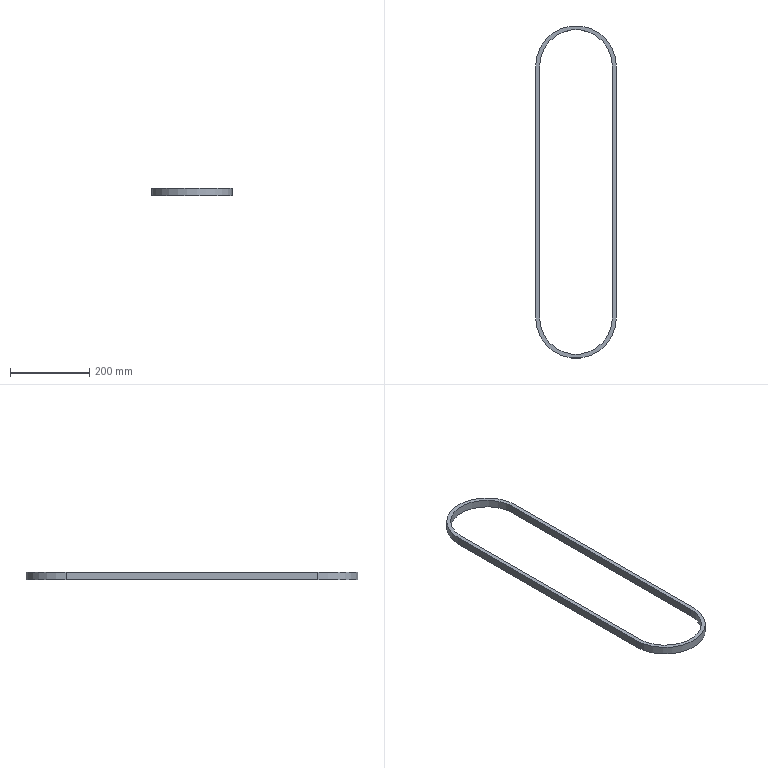Part | SolidWorks | features BeltProfileFeature 1, ExtruThin 1 | 1 solid | 10 faces | box 203.25 x 838.25 x 20 mm | volume 375423 mm3 | plane 6 | cylinder 4 | commonest cylinder face diameters 183.25 x2 203.25 x2
STEP:
#1=CARTESIAN_POINT('',(101.625,0.,10.));
#2=VERTEX_POINT('',#1);
#3=CARTESIAN_POINT('',(-101.625,0.,10.));
#4=VERTEX_POINT('',#3);
#5=CARTESIAN_POINT('',(0.,0.,10.));
#6=DIRECTION('',(0.,0.,1.));
#7=DIRECTION('',(-1.,0.,0.));
#8=AXIS2_PLACEMENT_3D('',#5,#6,#7);
#9=CIRCLE('',#8,101.625);
#10=EDGE_CURVE('',#2,#4,#9,.T.);
#11=ORIENTED_EDGE('',*,*,#10,.T.);
#12=CARTESIAN_POINT('',(-101.625,-635.,10.));
#13=VERTEX_POINT('',#12);
#14=CARTESIAN_POINT('',(-101.625,0.,10.));
#15=DIRECTION('',(0.,-1.,0.));
#16=VECTOR('',#15,1000.);
#17=LINE('',#14,#16);
#18=EDGE_CURVE('',#4,#13,#17,.T.);
#19=ORIENTED_EDGE('',*,*,#18,.T.);
#20=CARTESIAN_POINT('',(101.625,-635.,10.));
#21=VERTEX_POINT('',#20);
#22=CARTESIAN_POINT('',(0.,-635.,10.));
#23=DIRECTION('',(0.,0.,1.));
#24=DIRECTION('',(-1.,0.,0.));
#25=AXIS2_PLACEMENT_3D('',#22,#23,#24);
#26=CIRCLE('',#25,101.625);
#27=EDGE_CURVE('',#13,#21,#26,.T.);
#28=ORIENTED_EDGE('',*,*,#27,.T.);
#29=CARTESIAN_POINT('',(101.625,0.,10.));
#30=DIRECTION('',(0.,1.,0.));
#31=VECTOR('',#30,1000.);
#32=LINE('',#29,#31);
#33=EDGE_CURVE('',#21,#2,#32,.T.);
#34=ORIENTED_EDGE('',*,*,#33,.T.);
#35=EDGE_LOOP('',(#11,#19,#28,#34));
#36=FACE_OUTER_BOUND('',#35,.T.);
#37=CARTESIAN_POINT('',(91.625,0.,10.));
#38=VERTEX_POINT('',#37);
#39=CARTESIAN_POINT('',(-91.625,0.,10.));
#40=VERTEX_POINT('',#39);
#41=CARTESIAN_POINT('',(0.,0.,10.));
#42=DIRECTION('',(0.,0.,1.));
#43=DIRECTION('',(-1.,0.,0.));
#44=AXIS2_PLACEMENT_3D('',#41,#42,#43);
#45=CIRCLE('',#44,91.625);
#46=EDGE_CURVE('',#38,#40,#45,.T.);
#47=ORIENTED_EDGE('',*,*,#46,.F.);
#48=CARTESIAN_POINT('',(91.625,-635.,10.));
#49=VERTEX_POINT('',#48);
#50=CARTESIAN_POINT('',(91.625,0.,10.));
#51=DIRECTION('',(0.,1.,0.));
#52=VECTOR('',#51,1000.);
#53=LINE('',#50,#52);
#54=EDGE_CURVE('',#49,#38,#53,.T.);
#55=ORIENTED_EDGE('',*,*,#54,.F.);
#56=CARTESIAN_POINT('',(-91.625,-635.,10.));
#57=VERTEX_POINT('',#56);
#58=CARTESIAN_POINT('',(0.,-635.,10.));
#59=DIRECTION('',(0.,0.,1.));
#60=DIRECTION('',(-1.,0.,0.));
#61=AXIS2_PLACEMENT_3D('',#58,#59,#60);
#62=CIRCLE('',#61,91.625);
#63=EDGE_CURVE('',#57,#49,#62,.T.);
#64=ORIENTED_EDGE('',*,*,#63,.F.);
#65=CARTESIAN_POINT('',(-91.625,-635.,10.));
#66=DIRECTION('',(0.,-1.,0.));
#67=VECTOR('',#66,1000.);
#68=LINE('',#65,#67);
#69=EDGE_CURVE('',#40,#57,#68,.T.);
#70=ORIENTED_EDGE('',*,*,#69,.F.);
#71=EDGE_LOOP('',(#47,#55,#64,#70));
#72=FACE_BOUND('',#71,.T.);
#73=CARTESIAN_POINT('',(0.,0.,10.));
#74=DIRECTION('',(0.,0.,-1.));
#75=DIRECTION('',(-1.,0.,0.));
#76=AXIS2_PLACEMENT_3D('',#73,#74,#75);
#77=PLANE('',#76);
#78=ADVANCED_FACE('',(#36,#72),#77,.F.);
#79=CARTESIAN_POINT('',(101.625,0.,-10.));
#80=VERTEX_POINT('',#79);
#81=CARTESIAN_POINT('',(-101.625,0.,-10.));
#82=VERTEX_POINT('',#81);
#83=CARTESIAN_POINT('',(0.,0.,-10.));
#84=DIRECTION('',(0.,0.,1.));
#85=DIRECTION('',(-1.,0.,0.));
#86=AXIS2_PLACEMENT_3D('',#83,#84,#85);
#87=CIRCLE('',#86,101.625);
#88=EDGE_CURVE('',#80,#82,#87,.T.);
#89=ORIENTED_EDGE('',*,*,#88,.F.);
#90=CARTESIAN_POINT('',(101.625,-635.,-10.));
#91=VERTEX_POINT('',#90);
#92=CARTESIAN_POINT('',(101.625,0.,-10.));
#93=DIRECTION('',(0.,1.,0.));
#94=VECTOR('',#93,1000.);
#95=LINE('',#92,#94);
#96=EDGE_CURVE('',#91,#80,#95,.T.);
#97=ORIENTED_EDGE('',*,*,#96,.F.);
#98=CARTESIAN_POINT('',(-101.625,-635.,-10.));
#99=VERTEX_POINT('',#98);
#100=CARTESIAN_POINT('',(0.,-635.,-10.));
#101=DIRECTION('',(0.,0.,1.));
#102=DIRECTION('',(-1.,0.,0.));
#103=AXIS2_PLACEMENT_3D('',#100,#101,#102);
#104=CIRCLE('',#103,101.625);
#105=EDGE_CURVE('',#99,#91,#104,.T.);
#106=ORIENTED_EDGE('',*,*,#105,.F.);
#107=CARTESIAN_POINT('',(-101.625,0.,-10.));
#108=DIRECTION('',(0.,-1.,0.));
#109=VECTOR('',#108,1000.);
#110=LINE('',#107,#109);
#111=EDGE_CURVE('',#82,#99,#110,.T.);
#112=ORIENTED_EDGE('',*,*,#111,.F.);
#113=EDGE_LOOP('',(#89,#97,#106,#112));
#114=FACE_OUTER_BOUND('',#113,.T.);
#115=CARTESIAN_POINT('',(91.625,-635.,-10.));
#116=VERTEX_POINT('',#115);
#117=CARTESIAN_POINT('',(91.625,0.,-10.));
#118=VERTEX_POINT('',#117);
#119=CARTESIAN_POINT('',(91.625,0.,-10.));
#120=DIRECTION('',(0.,1.,0.));
#121=VECTOR('',#120,1000.);
#122=LINE('',#119,#121);
#123=EDGE_CURVE('',#116,#118,#122,.T.);
#124=ORIENTED_EDGE('',*,*,#123,.T.);
#125=CARTESIAN_POINT('',(-91.625,0.,-10.));
#126=VERTEX_POINT('',#125);
#127=CARTESIAN_POINT('',(0.,0.,-10.));
#128=DIRECTION('',(0.,0.,1.));
#129=DIRECTION('',(-1.,0.,0.));
#130=AXIS2_PLACEMENT_3D('',#127,#128,#129);
#131=CIRCLE('',#130,91.625);
#132=EDGE_CURVE('',#118,#126,#131,.T.);
#133=ORIENTED_EDGE('',*,*,#132,.T.);
#134=CARTESIAN_POINT('',(-91.625,-635.,-10.));
#135=VERTEX_POINT('',#134);
#136=CARTESIAN_POINT('',(-91.625,-635.,-10.));
#137=DIRECTION('',(0.,-1.,0.));
#138=VECTOR('',#137,1000.);
#139=LINE('',#136,#138);
#140=EDGE_CURVE('',#126,#135,#139,.T.);
#141=ORIENTED_EDGE('',*,*,#140,.T.);
#142=CARTESIAN_POINT('',(0.,-635.,-10.));
#143=DIRECTION('',(0.,0.,1.));
#144=DIRECTION('',(-1.,0.,0.));
#145=AXIS2_PLACEMENT_3D('',#142,#143,#144);
#146=CIRCLE('',#145,91.625);
#147=EDGE_CURVE('',#135,#116,#146,.T.);
#148=ORIENTED_EDGE('',*,*,#147,.T.);
#149=EDGE_LOOP('',(#124,#133,#141,#148));
#150=FACE_BOUND('',#149,.T.);
#151=CARTESIAN_POINT('',(0.,0.,-10.));
#152=DIRECTION('',(0.,0.,-1.));
#153=DIRECTION('',(-1.,0.,0.));
#154=AXIS2_PLACEMENT_3D('',#151,#152,#153);
#155=PLANE('',#154);
#156=ADVANCED_FACE('',(#114,#150),#155,.T.);
#157=ORIENTED_EDGE('',*,*,#88,.T.);
#158=CARTESIAN_POINT('',(-101.625,0.,10.));
#159=DIRECTION('',(0.,0.,-1.));
#160=VECTOR('',#159,1000.);
#161=LINE('',#158,#160);
#162=EDGE_CURVE('',#4,#82,#161,.T.);
#163=ORIENTED_EDGE('',*,*,#162,.F.);
#164=ORIENTED_EDGE('',*,*,#10,.F.);
#165=CARTESIAN_POINT('',(101.625,0.,10.));
#166=DIRECTION('',(0.,0.,-1.));
#167=VECTOR('',#166,1000.);
#168=LINE('',#165,#167);
#169=EDGE_CURVE('',#2,#80,#168,.T.);
#170=ORIENTED_EDGE('',*,*,#169,.T.);
#171=EDGE_LOOP('',(#157,#163,#164,#170));
#172=FACE_OUTER_BOUND('',#171,.T.);
#173=CARTESIAN_POINT('',(0.,0.,10.));
#174=DIRECTION('',(0.,0.,-1.));
#175=DIRECTION('',(-1.,0.,0.));
#176=AXIS2_PLACEMENT_3D('',#173,#174,#175);
#177=CYLINDRICAL_SURFACE('',#176,101.625);
#178=ADVANCED_FACE('',(#172),#177,.T.);
#179=ORIENTED_EDGE('',*,*,#111,.T.);
#180=CARTESIAN_POINT('',(-101.625,-635.,10.));
#181=DIRECTION('',(0.,0.,-1.));
#182=VECTOR('',#181,1000.);
#183=LINE('',#180,#182);
#184=EDGE_CURVE('',#13,#99,#183,.T.);
#185=ORIENTED_EDGE('',*,*,#184,.F.);
#186=ORIENTED_EDGE('',*,*,#18,.F.);
#187=ORIENTED_EDGE('',*,*,#162,.T.);
#188=EDGE_LOOP('',(#179,#185,#186,#187));
#189=FACE_OUTER_BOUND('',#188,.T.);
#190=CARTESIAN_POINT('',(-101.625,0.,10.));
#191=DIRECTION('',(1.,0.,0.));
#192=DIRECTION('',(0.,1.,0.));
#193=AXIS2_PLACEMENT_3D('',#190,#191,#192);
#194=PLANE('',#193);
#195=ADVANCED_FACE('',(#189),#194,.F.);
#196=ORIENTED_EDGE('',*,*,#105,.T.);
#197=CARTESIAN_POINT('',(101.625,-635.,10.));
#198=DIRECTION('',(0.,0.,-1.));
#199=VECTOR('',#198,1000.);
#200=LINE('',#197,#199);
#201=EDGE_CURVE('',#21,#91,#200,.T.);
#202=ORIENTED_EDGE('',*,*,#201,.F.);
#203=ORIENTED_EDGE('',*,*,#27,.F.);
#204=ORIENTED_EDGE('',*,*,#184,.T.);
#205=EDGE_LOOP('',(#196,#202,#203,#204));
#206=FACE_OUTER_BOUND('',#205,.T.);
#207=CARTESIAN_POINT('',(0.,-635.,10.));
#208=DIRECTION('',(0.,0.,-1.));
#209=DIRECTION('',(-1.,0.,0.));
#210=AXIS2_PLACEMENT_3D('',#207,#208,#209);
#211=CYLINDRICAL_SURFACE('',#210,101.625);
#212=ADVANCED_FACE('',(#206),#211,.T.);
#213=ORIENTED_EDGE('',*,*,#96,.T.);
#214=ORIENTED_EDGE('',*,*,#169,.F.);
#215=ORIENTED_EDGE('',*,*,#33,.F.);
#216=ORIENTED_EDGE('',*,*,#201,.T.);
#217=EDGE_LOOP('',(#213,#214,#215,#216));
#218=FACE_OUTER_BOUND('',#217,.T.);
#219=CARTESIAN_POINT('',(101.625,0.,10.));
#220=DIRECTION('',(-1.,0.,0.));
#221=DIRECTION('',(0.,-1.,0.));
#222=AXIS2_PLACEMENT_3D('',#219,#220,#221);
#223=PLANE('',#222);
#224=ADVANCED_FACE('',(#218),#223,.F.);
#225=ORIENTED_EDGE('',*,*,#132,.F.);
#226=CARTESIAN_POINT('',(91.625,0.,10.));
#227=DIRECTION('',(0.,0.,-1.));
#228=VECTOR('',#227,1000.);
#229=LINE('',#226,#228);
#230=EDGE_CURVE('',#38,#118,#229,.T.);
#231=ORIENTED_EDGE('',*,*,#230,.F.);
#232=ORIENTED_EDGE('',*,*,#46,.T.);
#233=CARTESIAN_POINT('',(-91.625,0.,10.));
#234=DIRECTION('',(0.,0.,-1.));
#235=VECTOR('',#234,1000.);
#236=LINE('',#233,#235);
#237=EDGE_CURVE('',#40,#126,#236,.T.);
#238=ORIENTED_EDGE('',*,*,#237,.T.);
#239=EDGE_LOOP('',(#225,#231,#232,#238));
#240=FACE_OUTER_BOUND('',#239,.T.);
#241=CARTESIAN_POINT('',(0.,0.,10.));
#242=DIRECTION('',(0.,0.,-1.));
#243=DIRECTION('',(-1.,0.,0.));
#244=AXIS2_PLACEMENT_3D('',#241,#242,#243);
#245=CYLINDRICAL_SURFACE('',#244,91.625);
#246=ADVANCED_FACE('',(#240),#245,.F.);
#247=ORIENTED_EDGE('',*,*,#140,.F.);
#248=ORIENTED_EDGE('',*,*,#237,.F.);
#249=ORIENTED_EDGE('',*,*,#69,.T.);
#250=CARTESIAN_POINT('',(-91.625,-635.,10.));
#251=DIRECTION('',(0.,0.,-1.));
#252=VECTOR('',#251,1000.);
#253=LINE('',#250,#252);
#254=EDGE_CURVE('',#57,#135,#253,.T.);
#255=ORIENTED_EDGE('',*,*,#254,.T.);
#256=EDGE_LOOP('',(#247,#248,#249,#255));
#257=FACE_OUTER_BOUND('',#256,.T.);
#258=CARTESIAN_POINT('',(-91.625,-635.,10.));
#259=DIRECTION('',(1.,0.,0.));
#260=DIRECTION('',(0.,1.,0.));
#261=AXIS2_PLACEMENT_3D('',#258,#259,#260);
#262=PLANE('',#261);
#263=ADVANCED_FACE('',(#257),#262,.T.);
#264=ORIENTED_EDGE('',*,*,#147,.F.);
#265=ORIENTED_EDGE('',*,*,#254,.F.);
#266=ORIENTED_EDGE('',*,*,#63,.T.);
#267=CARTESIAN_POINT('',(91.625,-635.,10.));
#268=DIRECTION('',(0.,0.,-1.));
#269=VECTOR('',#268,1000.);
#270=LINE('',#267,#269);
#271=EDGE_CURVE('',#49,#116,#270,.T.);
#272=ORIENTED_EDGE('',*,*,#271,.T.);
#273=EDGE_LOOP('',(#264,#265,#266,#272));
#274=FACE_OUTER_BOUND('',#273,.T.);
#275=CARTESIAN_POINT('',(0.,-635.,10.));
#276=DIRECTION('',(0.,0.,-1.));
#277=DIRECTION('',(-1.,0.,0.));
#278=AXIS2_PLACEMENT_3D('',#275,#276,#277);
#279=CYLINDRICAL_SURFACE('',#278,91.625);
#280=ADVANCED_FACE('',(#274),#279,.F.);
#281=ORIENTED_EDGE('',*,*,#123,.F.);
#282=ORIENTED_EDGE('',*,*,#271,.F.);
#283=ORIENTED_EDGE('',*,*,#54,.T.);
#284=ORIENTED_EDGE('',*,*,#230,.T.);
#285=EDGE_LOOP('',(#281,#282,#283,#284));
#286=FACE_OUTER_BOUND('',#285,.T.);
#287=CARTESIAN_POINT('',(91.625,0.,10.));
#288=DIRECTION('',(-1.,0.,0.));
#289=DIRECTION('',(0.,-1.,0.));
#290=AXIS2_PLACEMENT_3D('',#287,#288,#289);
#291=PLANE('',#290);
#292=ADVANCED_FACE('',(#286),#291,.T.);
#293=CLOSED_SHELL('',(#78,#156,#178,#195,#212,#224,#246,#263,#280,#292));
#294=MANIFOLD_SOLID_BREP('',#293);
#295=CARTESIAN_POINT('',(0.,0.,0.));
#296=DIRECTION('',(0.,0.,1.));
#297=DIRECTION('',(1.,0.,0.));
#298=AXIS2_PLACEMENT_3D('',#295,#296,#297);
#299=(LENGTH_UNIT()NAMED_UNIT(*)SI_UNIT(.MILLI.,.METRE.));
#300=UNCERTAINTY_MEASURE_WITH_UNIT(LENGTH_MEASURE(0.00001),#299,'','');
#301=(NAMED_UNIT(*)PLANE_ANGLE_UNIT()SI_UNIT($,.RADIAN.));
#302=(NAMED_UNIT(*)SI_UNIT($,.STERADIAN.)SOLID_ANGLE_UNIT());
#303=(GEOMETRIC_REPRESENTATION_CONTEXT(3)GLOBAL_UNCERTAINTY_ASSIGNED_CONTEXT((#300))GLOBAL_UNIT_ASSIGNED_CONTEXT((#299,#301,#302))REPRESENTATION_CONTEXT('',''));
#304=ADVANCED_BREP_SHAPE_REPRESENTATION('',(#294,#298),#303);